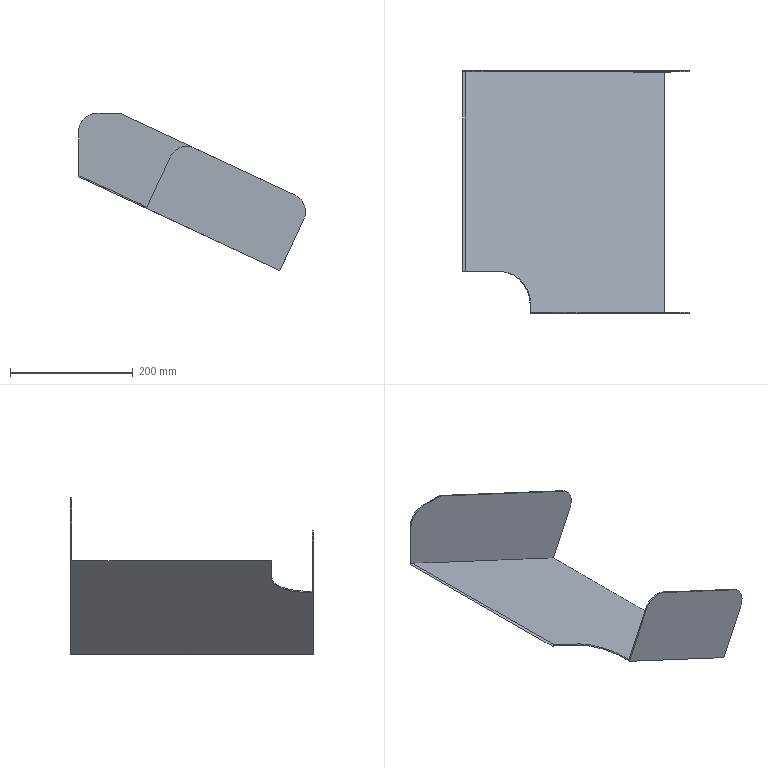Part | NX | features HB 2 | 1 solid | 19 faces | box 369.707 x 395.502 x 255.956 mm | volume 417373 mm3 | plane 14 | cylinder 5 | commonest cylinder face diameters 60 x4 110 x1
STEP:
#1=CARTESIAN_POINT('',(3925.845,2.,-162.6));
#2=VERTEX_POINT('',#1);
#3=CARTESIAN_POINT('',(4143.607,2.,-264.144));
#4=VERTEX_POINT('',#3);
#5=CARTESIAN_POINT('',(3774.845,2.,-92.187));
#6=DIRECTION('',(0.9063,0.,-0.4226));
#7=VECTOR('',#6,1000.);
#8=LINE('',#5,#7);
#9=EDGE_CURVE('',#2,#4,#8,.T.);
#10=ORIENTED_EDGE('',*,*,#9,.T.);
#11=CARTESIAN_POINT('',(4143.607,393.502,-264.144));
#12=VERTEX_POINT('',#11);
#13=CARTESIAN_POINT('',(4143.607,-399.,-264.144));
#14=DIRECTION('',(0.,1.,0.));
#15=VECTOR('',#14,1000.);
#16=LINE('',#13,#15);
#17=EDGE_CURVE('',#4,#12,#16,.T.);
#18=ORIENTED_EDGE('',*,*,#17,.T.);
#19=CARTESIAN_POINT('',(3819.478,393.502,-113.));
#20=VERTEX_POINT('',#19);
#21=CARTESIAN_POINT('',(3774.845,393.502,-92.187));
#22=DIRECTION('',(0.9063,0.,-0.4226));
#23=VECTOR('',#22,1000.);
#24=LINE('',#21,#23);
#25=EDGE_CURVE('',#20,#12,#24,.T.);
#26=ORIENTED_EDGE('',*,*,#25,.F.);
#27=CARTESIAN_POINT('',(3819.478,68.204,-113.));
#28=VERTEX_POINT('',#27);
#29=CARTESIAN_POINT('',(3819.478,399.,-113.));
#30=DIRECTION('',(0.,-1.,0.));
#31=VECTOR('',#30,1000.);
#32=LINE('',#29,#31);
#33=EDGE_CURVE('',#20,#28,#32,.T.);
#34=ORIENTED_EDGE('',*,*,#33,.T.);
#35=CARTESIAN_POINT('',(3875.998,68.204,-139.356));
#36=VERTEX_POINT('',#35);
#37=CARTESIAN_POINT('',(3774.845,68.204,-92.187));
#38=DIRECTION('',(-0.9063,0.,0.4226));
#39=VECTOR('',#38,1000.);
#40=LINE('',#37,#39);
#41=EDGE_CURVE('',#36,#28,#40,.T.);
#42=ORIENTED_EDGE('',*,*,#41,.F.);
#43=CARTESIAN_POINT('',(3925.845,13.204,-162.6));
#44=VERTEX_POINT('',#43);
#45=CARTESIAN_POINT('',(3875.998,13.204,-139.356));
#46=DIRECTION('',(0.4226,0.,0.9063));
#47=DIRECTION('',(-0.9063,0.,0.4226));
#48=AXIS2_PLACEMENT_3D('',#45,#46,#47);
#49=CIRCLE('',#48,55.);
#50=EDGE_CURVE('',#44,#36,#49,.T.);
#51=ORIENTED_EDGE('',*,*,#50,.F.);
#52=CARTESIAN_POINT('',(3925.845,-399.,-162.6));
#53=DIRECTION('',(0.,-1.,0.));
#54=VECTOR('',#53,1000.);
#55=LINE('',#52,#54);
#56=EDGE_CURVE('',#44,#2,#55,.T.);
#57=ORIENTED_EDGE('',*,*,#56,.T.);
#58=EDGE_LOOP('',(#10,#18,#26,#34,#42,#51,#57));
#59=FACE_BOUND('',#58,.T.);
#60=CARTESIAN_POINT('',(3774.845,-399.,-92.187));
#61=DIRECTION('',(-0.4226,0.,-0.9063));
#62=DIRECTION('',(0.9063,0.,-0.4226));
#63=AXIS2_PLACEMENT_3D('',#60,#61,#62);
#64=PLANE('',#63);
#65=ADVANCED_FACE('',(#59),#64,.F.);
#66=CARTESIAN_POINT('',(4142.761,0.,-265.956));
#67=VERTEX_POINT('',#66);
#68=CARTESIAN_POINT('',(4181.642,0.,-182.576));
#69=VERTEX_POINT('',#68);
#70=CARTESIAN_POINT('',(4168.611,0.,-210.52));
#71=DIRECTION('',(0.4226,0.,0.9063));
#72=VECTOR('',#71,1000.);
#73=LINE('',#70,#72);
#74=EDGE_CURVE('',#67,#69,#73,.T.);
#75=ORIENTED_EDGE('',*,*,#74,.F.);
#76=CARTESIAN_POINT('',(4142.761,395.502,-265.956));
#77=VERTEX_POINT('',#76);
#78=CARTESIAN_POINT('',(4142.761,-399.,-265.956));
#79=DIRECTION('',(0.,1.,0.));
#80=VECTOR('',#79,1000.);
#81=LINE('',#78,#80);
#82=EDGE_CURVE('',#67,#77,#81,.T.);
#83=ORIENTED_EDGE('',*,*,#82,.T.);
#84=CARTESIAN_POINT('',(4181.642,395.502,-182.576));
#85=VERTEX_POINT('',#84);
#86=CARTESIAN_POINT('',(4168.611,395.502,-210.52));
#87=DIRECTION('',(-0.4226,0.,-0.9063));
#88=VECTOR('',#87,1000.);
#89=LINE('',#86,#88);
#90=EDGE_CURVE('',#85,#77,#89,.T.);
#91=ORIENTED_EDGE('',*,*,#90,.F.);
#92=CARTESIAN_POINT('',(4181.642,393.502,-182.576));
#93=VERTEX_POINT('',#92);
#94=CARTESIAN_POINT('',(4181.642,-399.,-182.576));
#95=DIRECTION('',(0.,1.,0.));
#96=VECTOR('',#95,1000.);
#97=LINE('',#94,#96);
#98=EDGE_CURVE('',#93,#85,#97,.T.);
#99=ORIENTED_EDGE('',*,*,#98,.F.);
#100=CARTESIAN_POINT('',(4168.611,393.502,-210.52));
#101=DIRECTION('',(0.4226,0.,0.9063));
#102=VECTOR('',#101,1000.);
#103=LINE('',#100,#102);
#104=EDGE_CURVE('',#12,#93,#103,.T.);
#105=ORIENTED_EDGE('',*,*,#104,.F.);
#106=ORIENTED_EDGE('',*,*,#17,.F.);
#107=CARTESIAN_POINT('',(4181.642,2.,-182.576));
#108=VERTEX_POINT('',#107);
#109=CARTESIAN_POINT('',(4168.611,2.,-210.52));
#110=DIRECTION('',(0.4226,0.,0.9063));
#111=VECTOR('',#110,1000.);
#112=LINE('',#109,#111);
#113=EDGE_CURVE('',#4,#108,#112,.T.);
#114=ORIENTED_EDGE('',*,*,#113,.T.);
#115=CARTESIAN_POINT('',(4181.642,-399.,-182.576));
#116=DIRECTION('',(0.,1.,0.));
#117=VECTOR('',#116,1000.);
#118=LINE('',#115,#117);
#119=EDGE_CURVE('',#69,#108,#118,.T.);
#120=ORIENTED_EDGE('',*,*,#119,.F.);
#121=EDGE_LOOP('',(#75,#83,#91,#99,#105,#106,#114,#120));
#122=FACE_BOUND('',#121,.T.);
#123=CARTESIAN_POINT('',(4168.611,-399.,-210.52));
#124=DIRECTION('',(0.9063,0.,-0.4226));
#125=DIRECTION('',(0.4226,0.,0.9063));
#126=AXIS2_PLACEMENT_3D('',#123,#124,#125);
#127=PLANE('',#126);
#128=ADVANCED_FACE('',(#122),#127,.T.);
#129=ORIENTED_EDGE('',*,*,#82,.F.);
#130=CARTESIAN_POINT('',(3925.,0.,-164.412));
#131=VERTEX_POINT('',#130);
#132=CARTESIAN_POINT('',(3774.,0.,-94.));
#133=DIRECTION('',(0.9063,0.,-0.4226));
#134=VECTOR('',#133,1000.);
#135=LINE('',#132,#134);
#136=EDGE_CURVE('',#131,#67,#135,.T.);
#137=ORIENTED_EDGE('',*,*,#136,.F.);
#138=CARTESIAN_POINT('',(3925.,13.204,-164.412));
#139=VERTEX_POINT('',#138);
#140=CARTESIAN_POINT('',(3925.,-48.204,-164.412));
#141=DIRECTION('',(0.,1.,0.));
#142=VECTOR('',#141,1000.);
#143=LINE('',#140,#142);
#144=EDGE_CURVE('',#131,#139,#143,.T.);
#145=ORIENTED_EDGE('',*,*,#144,.T.);
#146=CARTESIAN_POINT('',(3875.153,68.204,-141.168));
#147=VERTEX_POINT('',#146);
#148=CARTESIAN_POINT('',(3875.153,13.204,-141.168));
#149=DIRECTION('',(-0.4226,0.,-0.9063));
#150=DIRECTION('',(-0.9063,0.,0.4226));
#151=AXIS2_PLACEMENT_3D('',#148,#149,#150);
#152=CIRCLE('',#151,55.);
#153=EDGE_CURVE('',#147,#139,#152,.T.);
#154=ORIENTED_EDGE('',*,*,#153,.F.);
#155=CARTESIAN_POINT('',(3814.746,68.204,-113.));
#156=VERTEX_POINT('',#155);
#157=CARTESIAN_POINT('',(3774.,68.204,-94.));
#158=DIRECTION('',(-0.9063,0.,0.4226));
#159=VECTOR('',#158,1000.);
#160=LINE('',#157,#159);
#161=EDGE_CURVE('',#147,#156,#160,.T.);
#162=ORIENTED_EDGE('',*,*,#161,.T.);
#163=CARTESIAN_POINT('',(3814.746,393.502,-113.));
#164=VERTEX_POINT('',#163);
#165=CARTESIAN_POINT('',(3814.746,399.,-113.));
#166=DIRECTION('',(0.,-1.,0.));
#167=VECTOR('',#166,1000.);
#168=LINE('',#165,#167);
#169=EDGE_CURVE('',#164,#156,#168,.T.);
#170=ORIENTED_EDGE('',*,*,#169,.F.);
#171=CARTESIAN_POINT('',(3814.746,395.502,-113.));
#172=VERTEX_POINT('',#171);
#173=CARTESIAN_POINT('',(3814.746,399.,-113.));
#174=DIRECTION('',(0.,-1.,0.));
#175=VECTOR('',#174,1000.);
#176=LINE('',#173,#175);
#177=EDGE_CURVE('',#172,#164,#176,.T.);
#178=ORIENTED_EDGE('',*,*,#177,.F.);
#179=CARTESIAN_POINT('',(3774.,395.502,-94.));
#180=DIRECTION('',(-0.9063,0.,0.4226));
#181=VECTOR('',#180,1000.);
#182=LINE('',#179,#181);
#183=EDGE_CURVE('',#77,#172,#182,.T.);
#184=ORIENTED_EDGE('',*,*,#183,.F.);
#185=EDGE_LOOP('',(#129,#137,#145,#154,#162,#170,#178,#184));
#186=FACE_BOUND('',#185,.T.);
#187=CARTESIAN_POINT('',(3774.,-399.,-94.));
#188=DIRECTION('',(-0.4226,0.,-0.9063));
#189=DIRECTION('',(0.9063,0.,-0.4226));
#190=AXIS2_PLACEMENT_3D('',#187,#188,#189);
#191=PLANE('',#190);
#192=ADVANCED_FACE('',(#186),#191,.T.);
#193=ORIENTED_EDGE('',*,*,#56,.F.);
#194=CARTESIAN_POINT('',(3914.524,13.204,-186.879));
#195=DIRECTION('',(0.4226,0.,0.9063));
#196=VECTOR('',#195,1000.);
#197=LINE('',#194,#196);
#198=EDGE_CURVE('',#139,#44,#197,.T.);
#199=ORIENTED_EDGE('',*,*,#198,.F.);
#200=ORIENTED_EDGE('',*,*,#144,.F.);
#201=CARTESIAN_POINT('',(3963.881,0.,-81.032));
#202=VERTEX_POINT('',#201);
#203=CARTESIAN_POINT('',(3925.,0.,-164.412));
#204=DIRECTION('',(0.4226,0.,0.9063));
#205=VECTOR('',#204,1000.);
#206=LINE('',#203,#205);
#207=EDGE_CURVE('',#131,#202,#206,.T.);
#208=ORIENTED_EDGE('',*,*,#207,.T.);
#209=CARTESIAN_POINT('',(3963.881,2.,-81.032));
#210=VERTEX_POINT('',#209);
#211=CARTESIAN_POINT('',(3963.881,-48.204,-81.032));
#212=DIRECTION('',(0.,-1.,0.));
#213=VECTOR('',#212,1000.);
#214=LINE('',#211,#213);
#215=EDGE_CURVE('',#210,#202,#214,.T.);
#216=ORIENTED_EDGE('',*,*,#215,.F.);
#217=CARTESIAN_POINT('',(3925.,2.,-164.412));
#218=DIRECTION('',(0.4226,0.,0.9063));
#219=VECTOR('',#218,1000.);
#220=LINE('',#217,#219);
#221=EDGE_CURVE('',#2,#210,#220,.T.);
#222=ORIENTED_EDGE('',*,*,#221,.F.);
#223=EDGE_LOOP('',(#193,#199,#200,#208,#216,#222));
#224=FACE_BOUND('',#223,.T.);
#225=CARTESIAN_POINT('',(3925.,-48.204,-164.412));
#226=DIRECTION('',(0.9063,0.,-0.4226));
#227=DIRECTION('',(0.4226,0.,0.9063));
#228=AXIS2_PLACEMENT_3D('',#225,#226,#227);
#229=PLANE('',#228);
#230=ADVANCED_FACE('',(#224),#229,.F.);
#231=ORIENTED_EDGE('',*,*,#90,.T.);
#232=ORIENTED_EDGE('',*,*,#183,.T.);
#233=CARTESIAN_POINT('',(3814.746,395.502,-40.));
#234=VERTEX_POINT('',#233);
#235=CARTESIAN_POINT('',(3814.746,395.502,-92.187));
#236=DIRECTION('',(0.,0.,-1.));
#237=VECTOR('',#236,1000.);
#238=LINE('',#235,#237);
#239=EDGE_CURVE('',#234,#172,#238,.T.);
#240=ORIENTED_EDGE('',*,*,#239,.F.);
#241=CARTESIAN_POINT('',(3844.746,395.502,-10.));
#242=VERTEX_POINT('',#241);
#243=CARTESIAN_POINT('',(3844.746,395.502,-40.));
#244=DIRECTION('',(0.,-1.,0.));
#245=DIRECTION('',(0.,0.,-1.));
#246=AXIS2_PLACEMENT_3D('',#243,#244,#245);
#247=CIRCLE('',#246,30.);
#248=EDGE_CURVE('',#242,#234,#247,.T.);
#249=ORIENTED_EDGE('',*,*,#248,.F.);
#250=CARTESIAN_POINT('',(3882.538,395.502,-10.));
#251=VERTEX_POINT('',#250);
#252=CARTESIAN_POINT('',(3598.,395.502,-10.));
#253=DIRECTION('',(-1.,0.,0.));
#254=VECTOR('',#253,1000.);
#255=LINE('',#252,#254);
#256=EDGE_CURVE('',#251,#242,#255,.T.);
#257=ORIENTED_EDGE('',*,*,#256,.F.);
#258=CARTESIAN_POINT('',(4167.132,395.502,-142.708));
#259=VERTEX_POINT('',#258);
#260=CARTESIAN_POINT('',(3825.559,395.502,16.57));
#261=DIRECTION('',(-0.9063,0.,0.4226));
#262=VECTOR('',#261,1000.);
#263=LINE('',#260,#262);
#264=EDGE_CURVE('',#259,#251,#263,.T.);
#265=ORIENTED_EDGE('',*,*,#264,.F.);
#266=CARTESIAN_POINT('',(4154.453,395.502,-169.897));
#267=DIRECTION('',(0.,-1.,0.));
#268=DIRECTION('',(0.,0.,-1.));
#269=AXIS2_PLACEMENT_3D('',#266,#267,#268);
#270=CIRCLE('',#269,30.);
#271=EDGE_CURVE('',#85,#259,#270,.T.);
#272=ORIENTED_EDGE('',*,*,#271,.F.);
#273=EDGE_LOOP('',(#231,#232,#240,#249,#257,#265,#272));
#274=FACE_BOUND('',#273,.T.);
#275=CARTESIAN_POINT('',(3774.845,395.502,-92.187));
#276=DIRECTION('',(0.,1.,0.));
#277=DIRECTION('',(0.,0.,1.));
#278=AXIS2_PLACEMENT_3D('',#275,#276,#277);
#279=PLANE('',#278);
#280=ADVANCED_FACE('',(#274),#279,.T.);
#281=CARTESIAN_POINT('',(4167.132,393.502,-142.708));
#282=VERTEX_POINT('',#281);
#283=CARTESIAN_POINT('',(3882.538,393.502,-10.));
#284=VERTEX_POINT('',#283);
#285=CARTESIAN_POINT('',(3973.162,393.502,-52.259));
#286=DIRECTION('',(-0.9063,0.,0.4226));
#287=VECTOR('',#286,1000.);
#288=LINE('',#285,#287);
#289=EDGE_CURVE('',#282,#284,#288,.T.);
#290=ORIENTED_EDGE('',*,*,#289,.T.);
#291=CARTESIAN_POINT('',(3844.746,393.502,-10.));
#292=VERTEX_POINT('',#291);
#293=CARTESIAN_POINT('',(3598.,393.502,-10.));
#294=DIRECTION('',(-1.,0.,0.));
#295=VECTOR('',#294,1000.);
#296=LINE('',#293,#295);
#297=EDGE_CURVE('',#284,#292,#296,.T.);
#298=ORIENTED_EDGE('',*,*,#297,.T.);
#299=CARTESIAN_POINT('',(3814.746,393.502,-40.));
#300=VERTEX_POINT('',#299);
#301=CARTESIAN_POINT('',(3844.746,393.502,-40.));
#302=DIRECTION('',(0.,1.,0.));
#303=DIRECTION('',(0.,0.,-1.));
#304=AXIS2_PLACEMENT_3D('',#301,#302,#303);
#305=CIRCLE('',#304,30.);
#306=EDGE_CURVE('',#300,#292,#305,.T.);
#307=ORIENTED_EDGE('',*,*,#306,.F.);
#308=CARTESIAN_POINT('',(3814.746,393.502,-162.667));
#309=DIRECTION('',(0.,0.,-1.));
#310=VECTOR('',#309,1000.);
#311=LINE('',#308,#310);
#312=EDGE_CURVE('',#300,#164,#311,.T.);
#313=ORIENTED_EDGE('',*,*,#312,.T.);
#314=CARTESIAN_POINT('',(3398.5,393.502,-113.));
#315=DIRECTION('',(1.,0.,0.));
#316=VECTOR('',#315,1000.);
#317=LINE('',#314,#316);
#318=EDGE_CURVE('',#164,#20,#317,.T.);
#319=ORIENTED_EDGE('',*,*,#318,.T.);
#320=ORIENTED_EDGE('',*,*,#25,.T.);
#321=ORIENTED_EDGE('',*,*,#104,.T.);
#322=CARTESIAN_POINT('',(4154.453,393.502,-169.897));
#323=DIRECTION('',(0.,1.,0.));
#324=DIRECTION('',(0.,0.,-1.));
#325=AXIS2_PLACEMENT_3D('',#322,#323,#324);
#326=CIRCLE('',#325,30.);
#327=EDGE_CURVE('',#282,#93,#326,.T.);
#328=ORIENTED_EDGE('',*,*,#327,.F.);
#329=EDGE_LOOP('',(#290,#298,#307,#313,#319,#320,#321,#328));
#330=FACE_BOUND('',#329,.T.);
#331=CARTESIAN_POINT('',(3921.679,393.502,-162.667));
#332=DIRECTION('',(0.,1.,0.));
#333=DIRECTION('',(0.,0.,1.));
#334=AXIS2_PLACEMENT_3D('',#331,#332,#333);
#335=PLANE('',#334);
#336=ADVANCED_FACE('',(#330),#335,.F.);
#337=CARTESIAN_POINT('',(3882.538,-193.,-10.));
#338=DIRECTION('',(0.,1.,0.));
#339=VECTOR('',#338,1000.);
#340=LINE('',#337,#339);
#341=EDGE_CURVE('',#284,#251,#340,.T.);
#342=ORIENTED_EDGE('',*,*,#341,.T.);
#343=ORIENTED_EDGE('',*,*,#256,.T.);
#344=CARTESIAN_POINT('',(3844.746,388.502,-10.));
#345=DIRECTION('',(0.,1.,0.));
#346=VECTOR('',#345,1000.);
#347=LINE('',#344,#346);
#348=EDGE_CURVE('',#292,#242,#347,.T.);
#349=ORIENTED_EDGE('',*,*,#348,.F.);
#350=ORIENTED_EDGE('',*,*,#297,.F.);
#351=EDGE_LOOP('',(#342,#343,#349,#350));
#352=FACE_BOUND('',#351,.T.);
#353=CARTESIAN_POINT('',(3598.,-193.,-10.));
#354=DIRECTION('',(0.,0.,1.));
#355=DIRECTION('',(0.,1.,0.));
#356=AXIS2_PLACEMENT_3D('',#353,#354,#355);
#357=PLANE('',#356);
#358=ADVANCED_FACE('',(#352),#357,.T.);
#359=ORIENTED_EDGE('',*,*,#33,.F.);
#360=ORIENTED_EDGE('',*,*,#318,.F.);
#361=ORIENTED_EDGE('',*,*,#169,.T.);
#362=CARTESIAN_POINT('',(3398.5,68.204,-113.));
#363=DIRECTION('',(-1.,0.,0.));
#364=VECTOR('',#363,1000.);
#365=LINE('',#362,#364);
#366=EDGE_CURVE('',#28,#156,#365,.T.);
#367=ORIENTED_EDGE('',*,*,#366,.F.);
#368=EDGE_LOOP('',(#359,#360,#361,#367));
#369=FACE_BOUND('',#368,.T.);
#370=CARTESIAN_POINT('',(3398.5,0.,-113.));
#371=DIRECTION('',(0.,0.,1.));
#372=DIRECTION('',(-1.,0.,0.));
#373=AXIS2_PLACEMENT_3D('',#370,#371,#372);
#374=PLANE('',#373);
#375=ADVANCED_FACE('',(#369),#374,.T.);
#376=ORIENTED_EDGE('',*,*,#239,.T.);
#377=ORIENTED_EDGE('',*,*,#177,.T.);
#378=ORIENTED_EDGE('',*,*,#312,.F.);
#379=CARTESIAN_POINT('',(3814.746,386.502,-40.));
#380=DIRECTION('',(0.,-1.,0.));
#381=VECTOR('',#380,1000.);
#382=LINE('',#379,#381);
#383=EDGE_CURVE('',#234,#300,#382,.T.);
#384=ORIENTED_EDGE('',*,*,#383,.F.);
#385=EDGE_LOOP('',(#376,#377,#378,#384));
#386=FACE_BOUND('',#385,.T.);
#387=CARTESIAN_POINT('',(3814.746,386.502,-113.));
#388=DIRECTION('',(-1.,0.,0.));
#389=DIRECTION('',(0.,0.,-1.));
#390=AXIS2_PLACEMENT_3D('',#387,#388,#389);
#391=PLANE('',#390);
#392=ADVANCED_FACE('',(#386),#391,.T.);
#393=CARTESIAN_POINT('',(3864.677,68.204,-163.635));
#394=DIRECTION('',(0.4226,0.,0.9063));
#395=VECTOR('',#394,1000.);
#396=LINE('',#393,#395);
#397=EDGE_CURVE('',#147,#36,#396,.T.);
#398=ORIENTED_EDGE('',*,*,#397,.T.);
#399=ORIENTED_EDGE('',*,*,#41,.T.);
#400=ORIENTED_EDGE('',*,*,#366,.T.);
#401=ORIENTED_EDGE('',*,*,#161,.F.);
#402=EDGE_LOOP('',(#398,#399,#400,#401));
#403=FACE_BOUND('',#402,.T.);
#404=CARTESIAN_POINT('',(3847.231,68.204,-155.5));
#405=DIRECTION('',(0.,-1.,0.));
#406=DIRECTION('',(0.,0.,-1.));
#407=AXIS2_PLACEMENT_3D('',#404,#405,#406);
#408=PLANE('',#407);
#409=ADVANCED_FACE('',(#403),#408,.T.);
#410=ORIENTED_EDGE('',*,*,#153,.T.);
#411=ORIENTED_EDGE('',*,*,#198,.T.);
#412=ORIENTED_EDGE('',*,*,#50,.T.);
#413=ORIENTED_EDGE('',*,*,#397,.F.);
#414=EDGE_LOOP('',(#410,#411,#412,#413));
#415=FACE_BOUND('',#414,.T.);
#416=CARTESIAN_POINT('',(3864.677,13.204,-163.635));
#417=DIRECTION('',(-0.4226,0.,-0.9063));
#418=DIRECTION('',(0.9063,0.,-0.4226));
#419=AXIS2_PLACEMENT_3D('',#416,#417,#418);
#420=CYLINDRICAL_SURFACE('',#419,55.);
#421=ADVANCED_FACE('',(#415),#420,.F.);
#422=ORIENTED_EDGE('',*,*,#306,.T.);
#423=ORIENTED_EDGE('',*,*,#348,.T.);
#424=ORIENTED_EDGE('',*,*,#248,.T.);
#425=ORIENTED_EDGE('',*,*,#383,.T.);
#426=EDGE_LOOP('',(#422,#423,#424,#425));
#427=FACE_BOUND('',#426,.T.);
#428=CARTESIAN_POINT('',(3844.746,-193.,-40.));
#429=DIRECTION('',(0.,1.,0.));
#430=DIRECTION('',(0.,0.,1.));
#431=AXIS2_PLACEMENT_3D('',#428,#429,#430);
#432=CYLINDRICAL_SURFACE('',#431,30.);
#433=ADVANCED_FACE('',(#427),#432,.T.);
#434=ORIENTED_EDGE('',*,*,#264,.T.);
#435=ORIENTED_EDGE('',*,*,#341,.F.);
#436=ORIENTED_EDGE('',*,*,#289,.F.);
#437=CARTESIAN_POINT('',(4167.132,0.,-142.708));
#438=DIRECTION('',(0.,-1.,0.));
#439=VECTOR('',#438,1000.);
#440=LINE('',#437,#439);
#441=EDGE_CURVE('',#259,#282,#440,.T.);
#442=ORIENTED_EDGE('',*,*,#441,.F.);
#443=EDGE_LOOP('',(#434,#435,#436,#442));
#444=FACE_BOUND('',#443,.T.);
#445=CARTESIAN_POINT('',(4032.256,0.,-79.815));
#446=DIRECTION('',(0.4226,0.,0.9063));
#447=DIRECTION('',(-0.9063,0.,0.4226));
#448=AXIS2_PLACEMENT_3D('',#445,#446,#447);
#449=PLANE('',#448);
#450=ADVANCED_FACE('',(#444),#449,.T.);
#451=ORIENTED_EDGE('',*,*,#327,.T.);
#452=ORIENTED_EDGE('',*,*,#98,.T.);
#453=ORIENTED_EDGE('',*,*,#271,.T.);
#454=ORIENTED_EDGE('',*,*,#441,.T.);
#455=EDGE_LOOP('',(#451,#452,#453,#454));
#456=FACE_BOUND('',#455,.T.);
#457=CARTESIAN_POINT('',(4154.453,-399.,-169.897));
#458=DIRECTION('',(0.,1.,0.));
#459=DIRECTION('',(0.,0.,1.));
#460=AXIS2_PLACEMENT_3D('',#457,#458,#459);
#461=CYLINDRICAL_SURFACE('',#460,30.);
#462=ADVANCED_FACE('',(#456),#461,.T.);
#463=ORIENTED_EDGE('',*,*,#74,.T.);
#464=CARTESIAN_POINT('',(4167.132,0.,-142.708));
#465=VERTEX_POINT('',#464);
#466=CARTESIAN_POINT('',(4154.453,0.,-169.897));
#467=DIRECTION('',(0.,1.,0.));
#468=DIRECTION('',(0.,0.,1.));
#469=AXIS2_PLACEMENT_3D('',#466,#467,#468);
#470=CIRCLE('',#469,30.);
#471=EDGE_CURVE('',#465,#69,#470,.T.);
#472=ORIENTED_EDGE('',*,*,#471,.F.);
#473=CARTESIAN_POINT('',(4003.749,0.,-66.521));
#474=VERTEX_POINT('',#473);
#475=CARTESIAN_POINT('',(689.615,0.,1478.884));
#476=DIRECTION('',(0.9063,0.,-0.4226));
#477=VECTOR('',#476,1000.);
#478=LINE('',#475,#477);
#479=EDGE_CURVE('',#474,#465,#478,.T.);
#480=ORIENTED_EDGE('',*,*,#479,.F.);
#481=CARTESIAN_POINT('',(3991.07,0.,-93.711));
#482=DIRECTION('',(0.,1.,0.));
#483=DIRECTION('',(0.,0.,1.));
#484=AXIS2_PLACEMENT_3D('',#481,#482,#483);
#485=CIRCLE('',#484,30.);
#486=EDGE_CURVE('',#202,#474,#485,.T.);
#487=ORIENTED_EDGE('',*,*,#486,.F.);
#488=ORIENTED_EDGE('',*,*,#207,.F.);
#489=ORIENTED_EDGE('',*,*,#136,.T.);
#490=EDGE_LOOP('',(#463,#472,#480,#487,#488,#489));
#491=FACE_BOUND('',#490,.T.);
#492=CARTESIAN_POINT('',(0.,0.,0.));
#493=DIRECTION('',(0.,-1.,0.));
#494=DIRECTION('',(0.,0.,-1.));
#495=AXIS2_PLACEMENT_3D('',#492,#493,#494);
#496=PLANE('',#495);
#497=ADVANCED_FACE('',(#491),#496,.T.);
#498=ORIENTED_EDGE('',*,*,#221,.T.);
#499=CARTESIAN_POINT('',(4003.749,2.,-66.521));
#500=VERTEX_POINT('',#499);
#501=CARTESIAN_POINT('',(3991.07,2.,-93.711));
#502=DIRECTION('',(0.,-1.,0.));
#503=DIRECTION('',(0.,0.,1.));
#504=AXIS2_PLACEMENT_3D('',#501,#502,#503);
#505=CIRCLE('',#504,30.);
#506=EDGE_CURVE('',#500,#210,#505,.T.);
#507=ORIENTED_EDGE('',*,*,#506,.F.);
#508=CARTESIAN_POINT('',(4167.132,2.,-142.708));
#509=VERTEX_POINT('',#508);
#510=CARTESIAN_POINT('',(689.615,2.,1478.884));
#511=DIRECTION('',(0.9063,0.,-0.4226));
#512=VECTOR('',#511,1000.);
#513=LINE('',#510,#512);
#514=EDGE_CURVE('',#500,#509,#513,.T.);
#515=ORIENTED_EDGE('',*,*,#514,.T.);
#516=CARTESIAN_POINT('',(4154.453,2.,-169.897));
#517=DIRECTION('',(0.,-1.,0.));
#518=DIRECTION('',(0.,0.,1.));
#519=AXIS2_PLACEMENT_3D('',#516,#517,#518);
#520=CIRCLE('',#519,30.);
#521=EDGE_CURVE('',#108,#509,#520,.T.);
#522=ORIENTED_EDGE('',*,*,#521,.F.);
#523=ORIENTED_EDGE('',*,*,#113,.F.);
#524=ORIENTED_EDGE('',*,*,#9,.F.);
#525=EDGE_LOOP('',(#498,#507,#515,#522,#523,#524));
#526=FACE_BOUND('',#525,.T.);
#527=CARTESIAN_POINT('',(0.,2.,0.));
#528=DIRECTION('',(0.,-1.,0.));
#529=DIRECTION('',(0.,0.,-1.));
#530=AXIS2_PLACEMENT_3D('',#527,#528,#529);
#531=PLANE('',#530);
#532=ADVANCED_FACE('',(#526),#531,.F.);
#533=ORIENTED_EDGE('',*,*,#514,.F.);
#534=CARTESIAN_POINT('',(4003.749,0.,-66.521));
#535=DIRECTION('',(0.,1.,0.));
#536=VECTOR('',#535,1000.);
#537=LINE('',#534,#536);
#538=EDGE_CURVE('',#474,#500,#537,.T.);
#539=ORIENTED_EDGE('',*,*,#538,.F.);
#540=ORIENTED_EDGE('',*,*,#479,.T.);
#541=CARTESIAN_POINT('',(4167.132,0.,-142.708));
#542=DIRECTION('',(0.,-1.,0.));
#543=VECTOR('',#542,1000.);
#544=LINE('',#541,#543);
#545=EDGE_CURVE('',#509,#465,#544,.T.);
#546=ORIENTED_EDGE('',*,*,#545,.F.);
#547=EDGE_LOOP('',(#533,#539,#540,#546));
#548=FACE_BOUND('',#547,.T.);
#549=CARTESIAN_POINT('',(4032.256,0.,-79.815));
#550=DIRECTION('',(0.4226,0.,0.9063));
#551=DIRECTION('',(-0.9063,0.,0.4226));
#552=AXIS2_PLACEMENT_3D('',#549,#550,#551);
#553=PLANE('',#552);
#554=ADVANCED_FACE('',(#548),#553,.T.);
#555=ORIENTED_EDGE('',*,*,#521,.T.);
#556=ORIENTED_EDGE('',*,*,#545,.T.);
#557=ORIENTED_EDGE('',*,*,#471,.T.);
#558=ORIENTED_EDGE('',*,*,#119,.T.);
#559=EDGE_LOOP('',(#555,#556,#557,#558));
#560=FACE_BOUND('',#559,.T.);
#561=CARTESIAN_POINT('',(4154.453,-399.,-169.897));
#562=DIRECTION('',(0.,1.,0.));
#563=DIRECTION('',(0.,0.,1.));
#564=AXIS2_PLACEMENT_3D('',#561,#562,#563);
#565=CYLINDRICAL_SURFACE('',#564,30.);
#566=ADVANCED_FACE('',(#560),#565,.T.);
#567=ORIENTED_EDGE('',*,*,#506,.T.);
#568=ORIENTED_EDGE('',*,*,#215,.T.);
#569=ORIENTED_EDGE('',*,*,#486,.T.);
#570=ORIENTED_EDGE('',*,*,#538,.T.);
#571=EDGE_LOOP('',(#567,#568,#569,#570));
#572=FACE_BOUND('',#571,.T.);
#573=CARTESIAN_POINT('',(3991.07,0.,-93.711));
#574=DIRECTION('',(0.,-1.,0.));
#575=DIRECTION('',(0.,0.,-1.));
#576=AXIS2_PLACEMENT_3D('',#573,#574,#575);
#577=CYLINDRICAL_SURFACE('',#576,30.);
#578=ADVANCED_FACE('',(#572),#577,.T.);
#579=CLOSED_SHELL('',(#65,#128,#192,#230,#280,#336,#358,#375,#392,#409,#421,#433,#450,#462,#497,#532,#554,#566,#578));
#580=MANIFOLD_SOLID_BREP('',#579);
#581=(LENGTH_UNIT()NAMED_UNIT(*)SI_UNIT(.MILLI.,.METRE.));
#582=UNCERTAINTY_MEASURE_WITH_UNIT(LENGTH_MEASURE(0.00001),#581,'','');
#583=(NAMED_UNIT(*)PLANE_ANGLE_UNIT()SI_UNIT($,.RADIAN.));
#584=(NAMED_UNIT(*)SI_UNIT($,.STERADIAN.)SOLID_ANGLE_UNIT());
#585=(GEOMETRIC_REPRESENTATION_CONTEXT(3)GLOBAL_UNCERTAINTY_ASSIGNED_CONTEXT((#582))GLOBAL_UNIT_ASSIGNED_CONTEXT((#581,#583,#584))REPRESENTATION_CONTEXT('',''));
#586=ADVANCED_BREP_SHAPE_REPRESENTATION('',(#580),#585);